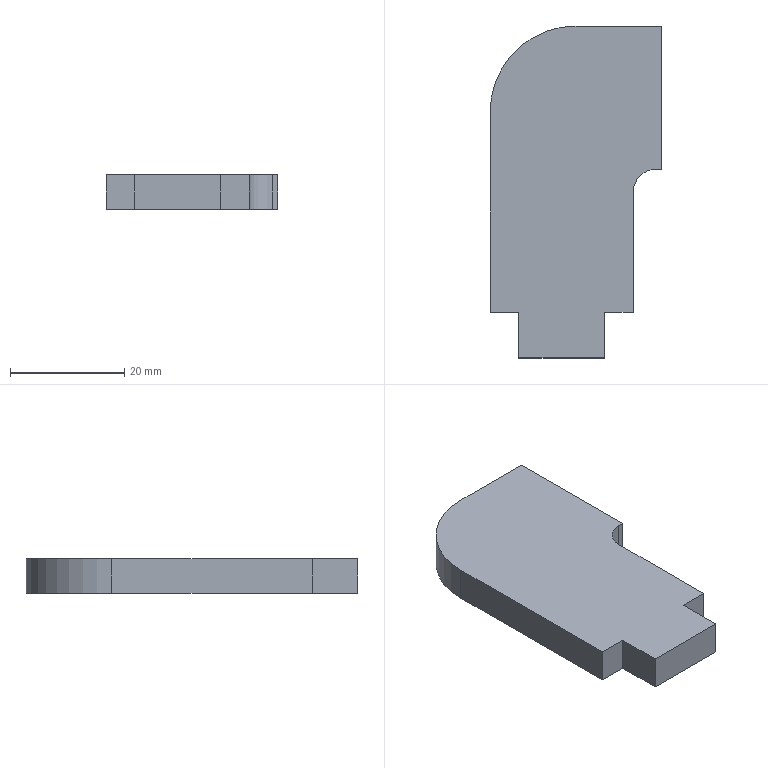Part | SolidWorks | features FlatPattern 1, SMBaseFlange 1, SheetMetal 1 | 1 solid | 14 faces | box 30 x 58 x 6 mm | volume 8701 mm3 | plane 12 | cylinder 2 | commonest cylinder face diameters 8 x1 30 x1
STEP:
#1=CARTESIAN_POINT('',(0.,-25.,0.));
#2=VERTEX_POINT('',#1);
#3=CARTESIAN_POINT('',(0.,0.,0.));
#4=VERTEX_POINT('',#3);
#5=CARTESIAN_POINT('',(0.,-25.,0.));
#6=DIRECTION('',(0.,1.,0.));
#7=VECTOR('',#6,1000.);
#8=LINE('',#5,#7);
#9=EDGE_CURVE('',#2,#4,#8,.T.);
#10=ORIENTED_EDGE('',*,*,#9,.T.);
#11=CARTESIAN_POINT('',(0.,0.,6.));
#12=VERTEX_POINT('',#11);
#13=CARTESIAN_POINT('',(0.,0.,6.));
#14=DIRECTION('',(0.,0.,-1.));
#15=VECTOR('',#14,1000.);
#16=LINE('',#13,#15);
#17=EDGE_CURVE('',#12,#4,#16,.T.);
#18=ORIENTED_EDGE('',*,*,#17,.F.);
#19=CARTESIAN_POINT('',(0.,-25.,6.));
#20=VERTEX_POINT('',#19);
#21=CARTESIAN_POINT('',(0.,-25.,6.));
#22=DIRECTION('',(0.,1.,0.));
#23=VECTOR('',#22,1000.);
#24=LINE('',#21,#23);
#25=EDGE_CURVE('',#20,#12,#24,.T.);
#26=ORIENTED_EDGE('',*,*,#25,.F.);
#27=CARTESIAN_POINT('',(0.,-25.,6.));
#28=DIRECTION('',(0.,0.,-1.));
#29=VECTOR('',#28,1000.);
#30=LINE('',#27,#29);
#31=EDGE_CURVE('',#20,#2,#30,.T.);
#32=ORIENTED_EDGE('',*,*,#31,.T.);
#33=EDGE_LOOP('',(#10,#18,#26,#32));
#34=FACE_OUTER_BOUND('',#33,.T.);
#35=CARTESIAN_POINT('',(0.,-25.,6.));
#36=DIRECTION('',(-1.,0.,0.));
#37=DIRECTION('',(0.,0.,1.));
#38=AXIS2_PLACEMENT_3D('',#35,#36,#37);
#39=PLANE('',#38);
#40=ADVANCED_FACE('',(#34),#39,.F.);
#41=CARTESIAN_POINT('',(-15.,0.,0.));
#42=VERTEX_POINT('',#41);
#43=CARTESIAN_POINT('',(0.,0.,0.));
#44=DIRECTION('',(-1.,0.,0.));
#45=VECTOR('',#44,1000.);
#46=LINE('',#43,#45);
#47=EDGE_CURVE('',#4,#42,#46,.T.);
#48=ORIENTED_EDGE('',*,*,#47,.T.);
#49=CARTESIAN_POINT('',(-15.,0.,6.));
#50=VERTEX_POINT('',#49);
#51=CARTESIAN_POINT('',(-15.,0.,6.));
#52=DIRECTION('',(0.,0.,-1.));
#53=VECTOR('',#52,1000.);
#54=LINE('',#51,#53);
#55=EDGE_CURVE('',#50,#42,#54,.T.);
#56=ORIENTED_EDGE('',*,*,#55,.F.);
#57=CARTESIAN_POINT('',(0.,0.,6.));
#58=DIRECTION('',(-1.,0.,0.));
#59=VECTOR('',#58,1000.);
#60=LINE('',#57,#59);
#61=EDGE_CURVE('',#12,#50,#60,.T.);
#62=ORIENTED_EDGE('',*,*,#61,.F.);
#63=ORIENTED_EDGE('',*,*,#17,.T.);
#64=EDGE_LOOP('',(#48,#56,#62,#63));
#65=FACE_OUTER_BOUND('',#64,.T.);
#66=CARTESIAN_POINT('',(0.,0.,6.));
#67=DIRECTION('',(0.,-1.,0.));
#68=DIRECTION('',(1.,0.,0.));
#69=AXIS2_PLACEMENT_3D('',#66,#67,#68);
#70=PLANE('',#69);
#71=ADVANCED_FACE('',(#65),#70,.F.);
#72=CARTESIAN_POINT('',(-30.,-15.,0.));
#73=VERTEX_POINT('',#72);
#74=CARTESIAN_POINT('',(-15.,-15.,0.));
#75=DIRECTION('',(0.,0.,1.));
#76=DIRECTION('',(1.,0.,0.));
#77=AXIS2_PLACEMENT_3D('',#74,#75,#76);
#78=CIRCLE('',#77,15.);
#79=EDGE_CURVE('',#42,#73,#78,.T.);
#80=ORIENTED_EDGE('',*,*,#79,.T.);
#81=CARTESIAN_POINT('',(-30.,-15.,6.));
#82=VERTEX_POINT('',#81);
#83=CARTESIAN_POINT('',(-30.,-15.,6.));
#84=DIRECTION('',(0.,0.,-1.));
#85=VECTOR('',#84,1000.);
#86=LINE('',#83,#85);
#87=EDGE_CURVE('',#82,#73,#86,.T.);
#88=ORIENTED_EDGE('',*,*,#87,.F.);
#89=CARTESIAN_POINT('',(-15.,-15.,6.));
#90=DIRECTION('',(0.,0.,1.));
#91=DIRECTION('',(1.,0.,0.));
#92=AXIS2_PLACEMENT_3D('',#89,#90,#91);
#93=CIRCLE('',#92,15.);
#94=EDGE_CURVE('',#50,#82,#93,.T.);
#95=ORIENTED_EDGE('',*,*,#94,.F.);
#96=ORIENTED_EDGE('',*,*,#55,.T.);
#97=EDGE_LOOP('',(#80,#88,#95,#96));
#98=FACE_OUTER_BOUND('',#97,.T.);
#99=CARTESIAN_POINT('',(-15.,-15.,6.));
#100=DIRECTION('',(0.,0.,-1.));
#101=DIRECTION('',(-1.,0.,0.));
#102=AXIS2_PLACEMENT_3D('',#99,#100,#101);
#103=CYLINDRICAL_SURFACE('',#102,15.);
#104=ADVANCED_FACE('',(#98),#103,.T.);
#105=CARTESIAN_POINT('',(-30.,-50.,0.));
#106=VERTEX_POINT('',#105);
#107=CARTESIAN_POINT('',(-30.,-15.,0.));
#108=DIRECTION('',(0.,-1.,0.));
#109=VECTOR('',#108,1000.);
#110=LINE('',#107,#109);
#111=EDGE_CURVE('',#73,#106,#110,.T.);
#112=ORIENTED_EDGE('',*,*,#111,.T.);
#113=CARTESIAN_POINT('',(-30.,-50.,6.));
#114=VERTEX_POINT('',#113);
#115=CARTESIAN_POINT('',(-30.,-50.,6.));
#116=DIRECTION('',(0.,0.,-1.));
#117=VECTOR('',#116,1000.);
#118=LINE('',#115,#117);
#119=EDGE_CURVE('',#114,#106,#118,.T.);
#120=ORIENTED_EDGE('',*,*,#119,.F.);
#121=CARTESIAN_POINT('',(-30.,-15.,6.));
#122=DIRECTION('',(0.,-1.,0.));
#123=VECTOR('',#122,1000.);
#124=LINE('',#121,#123);
#125=EDGE_CURVE('',#82,#114,#124,.T.);
#126=ORIENTED_EDGE('',*,*,#125,.F.);
#127=ORIENTED_EDGE('',*,*,#87,.T.);
#128=EDGE_LOOP('',(#112,#120,#126,#127));
#129=FACE_OUTER_BOUND('',#128,.T.);
#130=CARTESIAN_POINT('',(-30.,-15.,6.));
#131=DIRECTION('',(1.,0.,0.));
#132=DIRECTION('',(0.,1.,0.));
#133=AXIS2_PLACEMENT_3D('',#130,#131,#132);
#134=PLANE('',#133);
#135=ADVANCED_FACE('',(#129),#134,.F.);
#136=CARTESIAN_POINT('',(-25.,-50.,0.));
#137=VERTEX_POINT('',#136);
#138=CARTESIAN_POINT('',(-30.,-50.,0.));
#139=DIRECTION('',(1.,0.,0.));
#140=VECTOR('',#139,1000.);
#141=LINE('',#138,#140);
#142=EDGE_CURVE('',#106,#137,#141,.T.);
#143=ORIENTED_EDGE('',*,*,#142,.T.);
#144=CARTESIAN_POINT('',(-25.,-50.,6.));
#145=VERTEX_POINT('',#144);
#146=CARTESIAN_POINT('',(-25.,-50.,6.));
#147=DIRECTION('',(0.,0.,-1.));
#148=VECTOR('',#147,1000.);
#149=LINE('',#146,#148);
#150=EDGE_CURVE('',#145,#137,#149,.T.);
#151=ORIENTED_EDGE('',*,*,#150,.F.);
#152=CARTESIAN_POINT('',(-30.,-50.,6.));
#153=DIRECTION('',(1.,0.,0.));
#154=VECTOR('',#153,1000.);
#155=LINE('',#152,#154);
#156=EDGE_CURVE('',#114,#145,#155,.T.);
#157=ORIENTED_EDGE('',*,*,#156,.F.);
#158=ORIENTED_EDGE('',*,*,#119,.T.);
#159=EDGE_LOOP('',(#143,#151,#157,#158));
#160=FACE_OUTER_BOUND('',#159,.T.);
#161=CARTESIAN_POINT('',(-30.,-50.,6.));
#162=DIRECTION('',(0.,1.,0.));
#163=DIRECTION('',(0.,0.,1.));
#164=AXIS2_PLACEMENT_3D('',#161,#162,#163);
#165=PLANE('',#164);
#166=ADVANCED_FACE('',(#160),#165,.F.);
#167=CARTESIAN_POINT('',(-25.,-58.,0.));
#168=VERTEX_POINT('',#167);
#169=CARTESIAN_POINT('',(-25.,-50.,0.));
#170=DIRECTION('',(0.,-1.,0.));
#171=VECTOR('',#170,1000.);
#172=LINE('',#169,#171);
#173=EDGE_CURVE('',#137,#168,#172,.T.);
#174=ORIENTED_EDGE('',*,*,#173,.T.);
#175=CARTESIAN_POINT('',(-25.,-58.,6.));
#176=VERTEX_POINT('',#175);
#177=CARTESIAN_POINT('',(-25.,-58.,6.));
#178=DIRECTION('',(0.,0.,-1.));
#179=VECTOR('',#178,1000.);
#180=LINE('',#177,#179);
#181=EDGE_CURVE('',#176,#168,#180,.T.);
#182=ORIENTED_EDGE('',*,*,#181,.F.);
#183=CARTESIAN_POINT('',(-25.,-50.,6.));
#184=DIRECTION('',(0.,-1.,0.));
#185=VECTOR('',#184,1000.);
#186=LINE('',#183,#185);
#187=EDGE_CURVE('',#145,#176,#186,.T.);
#188=ORIENTED_EDGE('',*,*,#187,.F.);
#189=ORIENTED_EDGE('',*,*,#150,.T.);
#190=EDGE_LOOP('',(#174,#182,#188,#189));
#191=FACE_OUTER_BOUND('',#190,.T.);
#192=CARTESIAN_POINT('',(-25.,-50.,6.));
#193=DIRECTION('',(1.,0.,0.));
#194=DIRECTION('',(0.,0.,-1.));
#195=AXIS2_PLACEMENT_3D('',#192,#193,#194);
#196=PLANE('',#195);
#197=ADVANCED_FACE('',(#191),#196,.F.);
#198=CARTESIAN_POINT('',(-10.,-58.,0.));
#199=VERTEX_POINT('',#198);
#200=CARTESIAN_POINT('',(-25.,-58.,0.));
#201=DIRECTION('',(1.,0.,0.));
#202=VECTOR('',#201,1000.);
#203=LINE('',#200,#202);
#204=EDGE_CURVE('',#168,#199,#203,.T.);
#205=ORIENTED_EDGE('',*,*,#204,.T.);
#206=CARTESIAN_POINT('',(-10.,-58.,6.));
#207=VERTEX_POINT('',#206);
#208=CARTESIAN_POINT('',(-10.,-58.,6.));
#209=DIRECTION('',(0.,0.,-1.));
#210=VECTOR('',#209,1000.);
#211=LINE('',#208,#210);
#212=EDGE_CURVE('',#207,#199,#211,.T.);
#213=ORIENTED_EDGE('',*,*,#212,.F.);
#214=CARTESIAN_POINT('',(-25.,-58.,6.));
#215=DIRECTION('',(1.,0.,0.));
#216=VECTOR('',#215,1000.);
#217=LINE('',#214,#216);
#218=EDGE_CURVE('',#176,#207,#217,.T.);
#219=ORIENTED_EDGE('',*,*,#218,.F.);
#220=ORIENTED_EDGE('',*,*,#181,.T.);
#221=EDGE_LOOP('',(#205,#213,#219,#220));
#222=FACE_OUTER_BOUND('',#221,.T.);
#223=CARTESIAN_POINT('',(-25.,-58.,6.));
#224=DIRECTION('',(0.,1.,0.));
#225=DIRECTION('',(0.,0.,1.));
#226=AXIS2_PLACEMENT_3D('',#223,#224,#225);
#227=PLANE('',#226);
#228=ADVANCED_FACE('',(#222),#227,.F.);
#229=CARTESIAN_POINT('',(-10.,-50.,0.));
#230=VERTEX_POINT('',#229);
#231=CARTESIAN_POINT('',(-10.,-58.,0.));
#232=DIRECTION('',(0.,1.,0.));
#233=VECTOR('',#232,1000.);
#234=LINE('',#231,#233);
#235=EDGE_CURVE('',#199,#230,#234,.T.);
#236=ORIENTED_EDGE('',*,*,#235,.T.);
#237=CARTESIAN_POINT('',(-10.,-50.,6.));
#238=VERTEX_POINT('',#237);
#239=CARTESIAN_POINT('',(-10.,-50.,6.));
#240=DIRECTION('',(0.,0.,-1.));
#241=VECTOR('',#240,1000.);
#242=LINE('',#239,#241);
#243=EDGE_CURVE('',#238,#230,#242,.T.);
#244=ORIENTED_EDGE('',*,*,#243,.F.);
#245=CARTESIAN_POINT('',(-10.,-58.,6.));
#246=DIRECTION('',(0.,1.,0.));
#247=VECTOR('',#246,1000.);
#248=LINE('',#245,#247);
#249=EDGE_CURVE('',#207,#238,#248,.T.);
#250=ORIENTED_EDGE('',*,*,#249,.F.);
#251=ORIENTED_EDGE('',*,*,#212,.T.);
#252=EDGE_LOOP('',(#236,#244,#250,#251));
#253=FACE_OUTER_BOUND('',#252,.T.);
#254=CARTESIAN_POINT('',(-10.,-58.,6.));
#255=DIRECTION('',(-1.,0.,0.));
#256=DIRECTION('',(0.,0.,1.));
#257=AXIS2_PLACEMENT_3D('',#254,#255,#256);
#258=PLANE('',#257);
#259=ADVANCED_FACE('',(#253),#258,.F.);
#260=CARTESIAN_POINT('',(-5.,-50.,0.));
#261=VERTEX_POINT('',#260);
#262=CARTESIAN_POINT('',(-10.,-50.,0.));
#263=DIRECTION('',(1.,0.,0.));
#264=VECTOR('',#263,1000.);
#265=LINE('',#262,#264);
#266=EDGE_CURVE('',#230,#261,#265,.T.);
#267=ORIENTED_EDGE('',*,*,#266,.T.);
#268=CARTESIAN_POINT('',(-5.,-50.,6.));
#269=VERTEX_POINT('',#268);
#270=CARTESIAN_POINT('',(-5.,-50.,6.));
#271=DIRECTION('',(0.,0.,-1.));
#272=VECTOR('',#271,1000.);
#273=LINE('',#270,#272);
#274=EDGE_CURVE('',#269,#261,#273,.T.);
#275=ORIENTED_EDGE('',*,*,#274,.F.);
#276=CARTESIAN_POINT('',(-10.,-50.,6.));
#277=DIRECTION('',(1.,0.,0.));
#278=VECTOR('',#277,1000.);
#279=LINE('',#276,#278);
#280=EDGE_CURVE('',#238,#269,#279,.T.);
#281=ORIENTED_EDGE('',*,*,#280,.F.);
#282=ORIENTED_EDGE('',*,*,#243,.T.);
#283=EDGE_LOOP('',(#267,#275,#281,#282));
#284=FACE_OUTER_BOUND('',#283,.T.);
#285=CARTESIAN_POINT('',(-10.,-50.,6.));
#286=DIRECTION('',(0.,1.,0.));
#287=DIRECTION('',(0.,0.,1.));
#288=AXIS2_PLACEMENT_3D('',#285,#286,#287);
#289=PLANE('',#288);
#290=ADVANCED_FACE('',(#284),#289,.F.);
#291=CARTESIAN_POINT('',(-5.,-29.,0.));
#292=VERTEX_POINT('',#291);
#293=CARTESIAN_POINT('',(-5.,-50.,0.));
#294=DIRECTION('',(0.,1.,0.));
#295=VECTOR('',#294,1000.);
#296=LINE('',#293,#295);
#297=EDGE_CURVE('',#261,#292,#296,.T.);
#298=ORIENTED_EDGE('',*,*,#297,.T.);
#299=CARTESIAN_POINT('',(-5.,-29.,6.));
#300=VERTEX_POINT('',#299);
#301=CARTESIAN_POINT('',(-5.,-29.,6.));
#302=DIRECTION('',(0.,0.,-1.));
#303=VECTOR('',#302,1000.);
#304=LINE('',#301,#303);
#305=EDGE_CURVE('',#300,#292,#304,.T.);
#306=ORIENTED_EDGE('',*,*,#305,.F.);
#307=CARTESIAN_POINT('',(-5.,-50.,6.));
#308=DIRECTION('',(0.,1.,0.));
#309=VECTOR('',#308,1000.);
#310=LINE('',#307,#309);
#311=EDGE_CURVE('',#269,#300,#310,.T.);
#312=ORIENTED_EDGE('',*,*,#311,.F.);
#313=ORIENTED_EDGE('',*,*,#274,.T.);
#314=EDGE_LOOP('',(#298,#306,#312,#313));
#315=FACE_OUTER_BOUND('',#314,.T.);
#316=CARTESIAN_POINT('',(-5.,-50.,6.));
#317=DIRECTION('',(-1.,0.,0.));
#318=DIRECTION('',(0.,-1.,0.));
#319=AXIS2_PLACEMENT_3D('',#316,#317,#318);
#320=PLANE('',#319);
#321=ADVANCED_FACE('',(#315),#320,.F.);
#322=CARTESIAN_POINT('',(-1.,-25.,0.));
#323=VERTEX_POINT('',#322);
#324=CARTESIAN_POINT('',(-1.,-29.,0.));
#325=DIRECTION('',(0.,0.,-1.));
#326=DIRECTION('',(-1.,0.,0.));
#327=AXIS2_PLACEMENT_3D('',#324,#325,#326);
#328=CIRCLE('',#327,4.);
#329=EDGE_CURVE('',#292,#323,#328,.T.);
#330=ORIENTED_EDGE('',*,*,#329,.T.);
#331=CARTESIAN_POINT('',(-1.,-25.,6.));
#332=VERTEX_POINT('',#331);
#333=CARTESIAN_POINT('',(-1.,-25.,6.));
#334=DIRECTION('',(0.,0.,-1.));
#335=VECTOR('',#334,1000.);
#336=LINE('',#333,#335);
#337=EDGE_CURVE('',#332,#323,#336,.T.);
#338=ORIENTED_EDGE('',*,*,#337,.F.);
#339=CARTESIAN_POINT('',(-1.,-29.,6.));
#340=DIRECTION('',(0.,0.,-1.));
#341=DIRECTION('',(-1.,0.,0.));
#342=AXIS2_PLACEMENT_3D('',#339,#340,#341);
#343=CIRCLE('',#342,4.);
#344=EDGE_CURVE('',#300,#332,#343,.T.);
#345=ORIENTED_EDGE('',*,*,#344,.F.);
#346=ORIENTED_EDGE('',*,*,#305,.T.);
#347=EDGE_LOOP('',(#330,#338,#345,#346));
#348=FACE_OUTER_BOUND('',#347,.T.);
#349=CARTESIAN_POINT('',(-1.,-29.,6.));
#350=DIRECTION('',(0.,0.,-1.));
#351=DIRECTION('',(-1.,0.,0.));
#352=AXIS2_PLACEMENT_3D('',#349,#350,#351);
#353=CYLINDRICAL_SURFACE('',#352,4.);
#354=ADVANCED_FACE('',(#348),#353,.F.);
#355=CARTESIAN_POINT('',(-1.,-25.,0.));
#356=DIRECTION('',(1.,0.,0.));
#357=VECTOR('',#356,1000.);
#358=LINE('',#355,#357);
#359=EDGE_CURVE('',#323,#2,#358,.T.);
#360=ORIENTED_EDGE('',*,*,#359,.T.);
#361=ORIENTED_EDGE('',*,*,#31,.F.);
#362=CARTESIAN_POINT('',(-1.,-25.,6.));
#363=DIRECTION('',(1.,0.,0.));
#364=VECTOR('',#363,1000.);
#365=LINE('',#362,#364);
#366=EDGE_CURVE('',#332,#20,#365,.T.);
#367=ORIENTED_EDGE('',*,*,#366,.F.);
#368=ORIENTED_EDGE('',*,*,#337,.T.);
#369=EDGE_LOOP('',(#360,#361,#367,#368));
#370=FACE_OUTER_BOUND('',#369,.T.);
#371=CARTESIAN_POINT('',(-1.,-25.,6.));
#372=DIRECTION('',(0.,1.,0.));
#373=DIRECTION('',(0.,0.,1.));
#374=AXIS2_PLACEMENT_3D('',#371,#372,#373);
#375=PLANE('',#374);
#376=ADVANCED_FACE('',(#370),#375,.F.);
#377=ORIENTED_EDGE('',*,*,#25,.T.);
#378=ORIENTED_EDGE('',*,*,#61,.T.);
#379=ORIENTED_EDGE('',*,*,#94,.T.);
#380=ORIENTED_EDGE('',*,*,#125,.T.);
#381=ORIENTED_EDGE('',*,*,#156,.T.);
#382=ORIENTED_EDGE('',*,*,#187,.T.);
#383=ORIENTED_EDGE('',*,*,#218,.T.);
#384=ORIENTED_EDGE('',*,*,#249,.T.);
#385=ORIENTED_EDGE('',*,*,#280,.T.);
#386=ORIENTED_EDGE('',*,*,#311,.T.);
#387=ORIENTED_EDGE('',*,*,#344,.T.);
#388=ORIENTED_EDGE('',*,*,#366,.T.);
#389=EDGE_LOOP('',(#377,#378,#379,#380,#381,#382,#383,#384,#385,#386,#387,#388));
#390=FACE_OUTER_BOUND('',#389,.T.);
#391=CARTESIAN_POINT('',(-15.,-15.,6.));
#392=DIRECTION('',(0.,0.,1.));
#393=DIRECTION('',(1.,0.,0.));
#394=AXIS2_PLACEMENT_3D('',#391,#392,#393);
#395=PLANE('',#394);
#396=ADVANCED_FACE('',(#390),#395,.T.);
#397=ORIENTED_EDGE('',*,*,#9,.F.);
#398=ORIENTED_EDGE('',*,*,#359,.F.);
#399=ORIENTED_EDGE('',*,*,#329,.F.);
#400=ORIENTED_EDGE('',*,*,#297,.F.);
#401=ORIENTED_EDGE('',*,*,#266,.F.);
#402=ORIENTED_EDGE('',*,*,#235,.F.);
#403=ORIENTED_EDGE('',*,*,#204,.F.);
#404=ORIENTED_EDGE('',*,*,#173,.F.);
#405=ORIENTED_EDGE('',*,*,#142,.F.);
#406=ORIENTED_EDGE('',*,*,#111,.F.);
#407=ORIENTED_EDGE('',*,*,#79,.F.);
#408=ORIENTED_EDGE('',*,*,#47,.F.);
#409=EDGE_LOOP('',(#397,#398,#399,#400,#401,#402,#403,#404,#405,#406,#407,#408));
#410=FACE_OUTER_BOUND('',#409,.T.);
#411=CARTESIAN_POINT('',(-15.,-15.,0.));
#412=DIRECTION('',(0.,0.,1.));
#413=DIRECTION('',(1.,0.,0.));
#414=AXIS2_PLACEMENT_3D('',#411,#412,#413);
#415=PLANE('',#414);
#416=ADVANCED_FACE('',(#410),#415,.F.);
#417=CLOSED_SHELL('',(#40,#71,#104,#135,#166,#197,#228,#259,#290,#321,#354,#376,#396,#416));
#418=MANIFOLD_SOLID_BREP('',#417);
#419=CARTESIAN_POINT('',(0.,0.,0.));
#420=DIRECTION('',(0.,0.,1.));
#421=DIRECTION('',(1.,0.,0.));
#422=AXIS2_PLACEMENT_3D('',#419,#420,#421);
#423=(LENGTH_UNIT()NAMED_UNIT(*)SI_UNIT(.MILLI.,.METRE.));
#424=UNCERTAINTY_MEASURE_WITH_UNIT(LENGTH_MEASURE(0.00001),#423,'','');
#425=(NAMED_UNIT(*)PLANE_ANGLE_UNIT()SI_UNIT($,.RADIAN.));
#426=(NAMED_UNIT(*)SI_UNIT($,.STERADIAN.)SOLID_ANGLE_UNIT());
#427=(GEOMETRIC_REPRESENTATION_CONTEXT(3)GLOBAL_UNCERTAINTY_ASSIGNED_CONTEXT((#424))GLOBAL_UNIT_ASSIGNED_CONTEXT((#423,#425,#426))REPRESENTATION_CONTEXT('',''));
#428=ADVANCED_BREP_SHAPE_REPRESENTATION('',(#418,#422),#427);